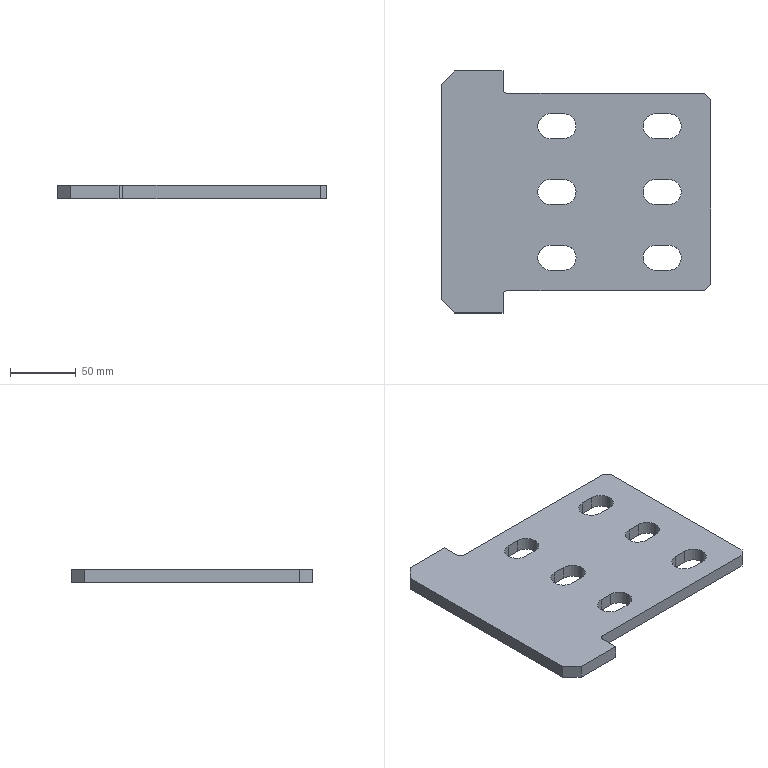Part | STEP file | 立柱腹Plate筋Plate-200×100-200 | 1 solid | 46 faces | box 205 x 184 x 10 mm | volume 293857 mm3 | plane 26 | cylinder 20 | commonest cylinder face diameters 19 x18 6 x2